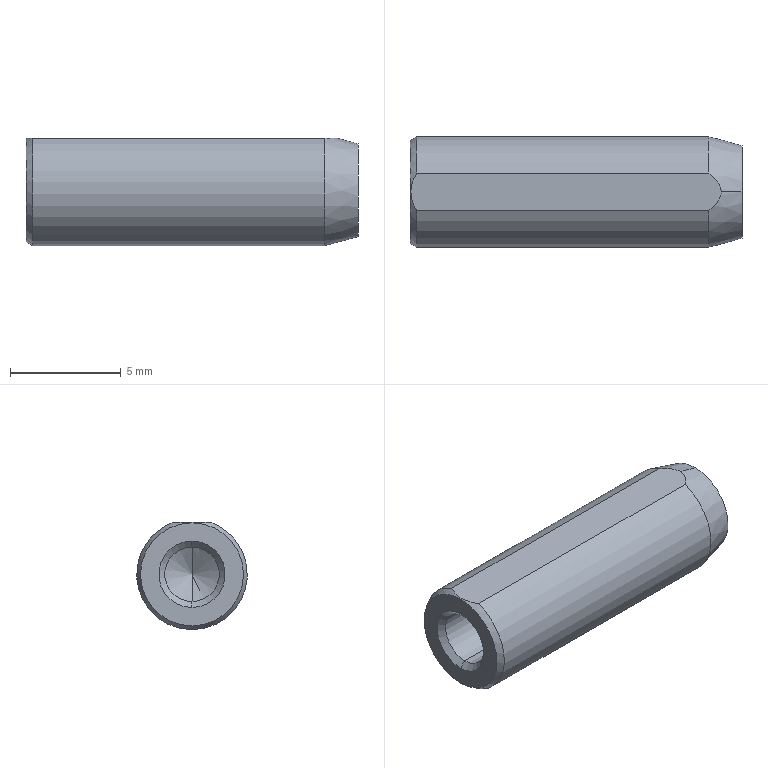Part | STEP file | MSTMS5-15-6 | 1 solid | 15 faces | box 15 x 5 x 4.85 mm | volume 252.224 mm3 | cone 8 | cylinder 4 | plane 3 | commonest cylinder face diameters 2.459 x2 5 x2
STEP:
#1=CARTESIAN_POINT('',(0.,0.,0.));
#2=DIRECTION('',(0.,0.,1.));
#3=DIRECTION('',(1.,0.,0.));
#4=AXIS2_PLACEMENT_3D('',#1,#2,#3);
#5=CARTESIAN_POINT('',(-0.4099,0.,1.23));
#6=VERTEX_POINT('',#5);
#7=CARTESIAN_POINT('',(-0.4099,0.,-1.23));
#8=VERTEX_POINT('',#7);
#9=CARTESIAN_POINT('',(-0.4099,0.,0.));
#10=DIRECTION('',(1.,0.,0.));
#11=DIRECTION('',(0.,0.,-1.));
#12=AXIS2_PLACEMENT_3D('',#9,#10,#11);
#13=CIRCLE('',#12,1.23);
#14=CARTESIAN_POINT('',(-0.4099,0.,0.));
#15=DIRECTION('',(-1.,0.,0.));
#16=DIRECTION('',(0.,0.,1.));
#17=AXIS2_PLACEMENT_3D('',#14,#15,#16);
#18=CONICAL_SURFACE('',#17,1.23,1.047);
#19=CARTESIAN_POINT('',(9.425,0.));
#20=DIRECTION('',(-1.,0.));
#21=VECTOR('',#20,1.);
#22=LINE('',#19,#21);
#23=(GEOMETRIC_REPRESENTATION_CONTEXT(2)PARAMETRIC_REPRESENTATION_CONTEXT()REPRESENTATION_CONTEXT('',''));
#24=DEFINITIONAL_REPRESENTATION('',(#22),#23);
#25=PCURVE('',#18,#24);
#26=CARTESIAN_POINT('',(0.3,0.,0.));
#27=DIRECTION('',(1.,0.,0.));
#28=DIRECTION('',(0.,0.,-1.));
#29=AXIS2_PLACEMENT_3D('',#26,#27,#28);
#30=CYLINDRICAL_SURFACE('',#29,1.23);
#31=CARTESIAN_POINT('',(0.,-0.7099));
#32=DIRECTION('',(1.,0.));
#33=VECTOR('',#32,1.);
#34=LINE('',#31,#33);
#35=(GEOMETRIC_REPRESENTATION_CONTEXT(2)PARAMETRIC_REPRESENTATION_CONTEXT()REPRESENTATION_CONTEXT('',''));
#36=DEFINITIONAL_REPRESENTATION('',(#34),#35);
#37=PCURVE('',#30,#36);
#38=SURFACE_CURVE('',#13,(#25,#37),.PCURVE_S1.);
#39=EDGE_CURVE('',#6,#8,#38,.T.);
#40=ORIENTED_EDGE('',*,*,#39,.T.);
#41=CARTESIAN_POINT('',(0.3,0.,0.));
#42=VERTEX_POINT('',#41);
#43=CARTESIAN_POINT('',(-0.4099,0.,-1.23));
#44=DIRECTION('',(-0.5,0.,-0.866));
#45=VECTOR('',#44,1.);
#46=LINE('',#43,#45);
#47=CARTESIAN_POINT('',(3.142,0.));
#48=DIRECTION('',(0.,1.));
#49=VECTOR('',#48,1.);
#50=LINE('',#47,#49);
#51=(GEOMETRIC_REPRESENTATION_CONTEXT(2)PARAMETRIC_REPRESENTATION_CONTEXT()REPRESENTATION_CONTEXT('',''));
#52=DEFINITIONAL_REPRESENTATION('',(#50),#51);
#53=PCURVE('',#18,#52);
#54=CARTESIAN_POINT('',(-0.4099,0.,0.));
#55=DIRECTION('',(-1.,0.,0.));
#56=DIRECTION('',(0.,0.,1.));
#57=AXIS2_PLACEMENT_3D('',#54,#55,#56);
#58=CONICAL_SURFACE('',#57,1.23,1.047);
#59=CARTESIAN_POINT('',(3.142,0.));
#60=DIRECTION('',(0.,1.));
#61=VECTOR('',#60,1.);
#62=LINE('',#59,#61);
#63=(GEOMETRIC_REPRESENTATION_CONTEXT(2)PARAMETRIC_REPRESENTATION_CONTEXT()REPRESENTATION_CONTEXT('',''));
#64=DEFINITIONAL_REPRESENTATION('',(#62),#63);
#65=PCURVE('',#58,#64);
#66=SURFACE_CURVE('',#46,(#53,#65),.PCURVE_S1.);
#67=EDGE_CURVE('',#42,#8,#66,.T.);
#68=ORIENTED_EDGE('',*,*,#67,.F.);
#69=CARTESIAN_POINT('',(-0.4099,0.,1.23));
#70=DIRECTION('',(-0.5,0.,0.866));
#71=VECTOR('',#70,1.);
#72=LINE('',#69,#71);
#73=CARTESIAN_POINT('',(6.283,0.));
#74=DIRECTION('',(0.,1.));
#75=VECTOR('',#74,1.);
#76=LINE('',#73,#75);
#77=(GEOMETRIC_REPRESENTATION_CONTEXT(2)PARAMETRIC_REPRESENTATION_CONTEXT()REPRESENTATION_CONTEXT('',''));
#78=DEFINITIONAL_REPRESENTATION('',(#76),#77);
#79=PCURVE('',#18,#78);
#80=CARTESIAN_POINT('',(0.,0.));
#81=DIRECTION('',(0.,1.));
#82=VECTOR('',#81,1.);
#83=LINE('',#80,#82);
#84=(GEOMETRIC_REPRESENTATION_CONTEXT(2)PARAMETRIC_REPRESENTATION_CONTEXT()REPRESENTATION_CONTEXT('',''));
#85=DEFINITIONAL_REPRESENTATION('',(#83),#84);
#86=PCURVE('',#58,#85);
#87=SURFACE_CURVE('',#72,(#79,#86),.PCURVE_S1.);
#88=EDGE_CURVE('',#42,#6,#87,.T.);
#89=ORIENTED_EDGE('',*,*,#88,.T.);
#90=EDGE_LOOP('',(#40,#68,#89));
#91=FACE_BOUND('',#90,.F.);
#92=ADVANCED_FACE('',(#91),#18,.F.);
#93=CARTESIAN_POINT('',(-7.229,0.,-1.23));
#94=VERTEX_POINT('',#93);
#95=CARTESIAN_POINT('',(0.3,0.,-1.23));
#96=DIRECTION('',(1.,0.,0.));
#97=VECTOR('',#96,1.);
#98=LINE('',#95,#97);
#99=CARTESIAN_POINT('',(6.283,0.));
#100=DIRECTION('',(0.,1.));
#101=VECTOR('',#100,1.);
#102=LINE('',#99,#101);
#103=(GEOMETRIC_REPRESENTATION_CONTEXT(2)PARAMETRIC_REPRESENTATION_CONTEXT()REPRESENTATION_CONTEXT('',''));
#104=DEFINITIONAL_REPRESENTATION('',(#102),#103);
#105=PCURVE('',#30,#104);
#106=CARTESIAN_POINT('',(0.3,0.,0.));
#107=DIRECTION('',(1.,0.,0.));
#108=DIRECTION('',(0.,0.,-1.));
#109=AXIS2_PLACEMENT_3D('',#106,#107,#108);
#110=CYLINDRICAL_SURFACE('',#109,1.23);
#111=CARTESIAN_POINT('',(0.,0.));
#112=DIRECTION('',(0.,1.));
#113=VECTOR('',#112,1.);
#114=LINE('',#111,#113);
#115=(GEOMETRIC_REPRESENTATION_CONTEXT(2)PARAMETRIC_REPRESENTATION_CONTEXT()REPRESENTATION_CONTEXT('',''));
#116=DEFINITIONAL_REPRESENTATION('',(#114),#115);
#117=PCURVE('',#110,#116);
#118=SURFACE_CURVE('',#98,(#105,#117),.PCURVE_S1.);
#119=EDGE_CURVE('',#94,#8,#118,.T.);
#120=ORIENTED_EDGE('',*,*,#119,.T.);
#121=ORIENTED_EDGE('',*,*,#39,.F.);
#122=CARTESIAN_POINT('',(-7.229,0.,1.23));
#123=VERTEX_POINT('',#122);
#124=CARTESIAN_POINT('',(0.3,0.,1.23));
#125=DIRECTION('',(1.,0.,0.));
#126=VECTOR('',#125,1.);
#127=LINE('',#124,#126);
#128=CARTESIAN_POINT('',(3.142,0.));
#129=DIRECTION('',(0.,1.));
#130=VECTOR('',#129,1.);
#131=LINE('',#128,#130);
#132=(GEOMETRIC_REPRESENTATION_CONTEXT(2)PARAMETRIC_REPRESENTATION_CONTEXT()REPRESENTATION_CONTEXT('',''));
#133=DEFINITIONAL_REPRESENTATION('',(#131),#132);
#134=PCURVE('',#30,#133);
#135=CARTESIAN_POINT('',(3.142,0.));
#136=DIRECTION('',(0.,1.));
#137=VECTOR('',#136,1.);
#138=LINE('',#135,#137);
#139=(GEOMETRIC_REPRESENTATION_CONTEXT(2)PARAMETRIC_REPRESENTATION_CONTEXT()REPRESENTATION_CONTEXT('',''));
#140=DEFINITIONAL_REPRESENTATION('',(#138),#139);
#141=PCURVE('',#110,#140);
#142=SURFACE_CURVE('',#127,(#134,#141),.PCURVE_S1.);
#143=EDGE_CURVE('',#123,#6,#142,.T.);
#144=ORIENTED_EDGE('',*,*,#143,.F.);
#145=CARTESIAN_POINT('',(-7.229,0.,0.));
#146=DIRECTION('',(1.,0.,0.));
#147=DIRECTION('',(0.,0.,-1.));
#148=AXIS2_PLACEMENT_3D('',#145,#146,#147);
#149=CIRCLE('',#148,1.23);
#150=CARTESIAN_POINT('',(0.,-7.529));
#151=DIRECTION('',(1.,0.));
#152=VECTOR('',#151,1.);
#153=LINE('',#150,#152);
#154=(GEOMETRIC_REPRESENTATION_CONTEXT(2)PARAMETRIC_REPRESENTATION_CONTEXT()REPRESENTATION_CONTEXT('',''));
#155=DEFINITIONAL_REPRESENTATION('',(#153),#154);
#156=PCURVE('',#30,#155);
#157=CARTESIAN_POINT('',(-7.5,0.,0.));
#158=DIRECTION('',(-1.,0.,0.));
#159=DIRECTION('',(0.,0.,1.));
#160=AXIS2_PLACEMENT_3D('',#157,#158,#159);
#161=CONICAL_SURFACE('',#160,1.5,0.7854);
#162=CARTESIAN_POINT('',(9.425,-0.2705));
#163=DIRECTION('',(-1.,0.));
#164=VECTOR('',#163,1.);
#165=LINE('',#162,#164);
#166=(GEOMETRIC_REPRESENTATION_CONTEXT(2)PARAMETRIC_REPRESENTATION_CONTEXT()REPRESENTATION_CONTEXT('',''));
#167=DEFINITIONAL_REPRESENTATION('',(#165),#166);
#168=PCURVE('',#161,#167);
#169=SURFACE_CURVE('',#149,(#156,#168),.PCURVE_S1.);
#170=EDGE_CURVE('',#123,#94,#169,.T.);
#171=ORIENTED_EDGE('',*,*,#170,.T.);
#172=EDGE_LOOP('',(#120,#121,#144,#171));
#173=FACE_BOUND('',#172,.F.);
#174=ADVANCED_FACE('',(#173),#30,.F.);
#175=CARTESIAN_POINT('',(-7.5,0.,1.5));
#176=VERTEX_POINT('',#175);
#177=CARTESIAN_POINT('',(-7.5,0.,1.5));
#178=DIRECTION('',(-0.7071,0.,0.7071));
#179=VECTOR('',#178,1.);
#180=LINE('',#177,#179);
#181=CARTESIAN_POINT('',(6.283,0.));
#182=DIRECTION('',(0.,1.));
#183=VECTOR('',#182,1.);
#184=LINE('',#181,#183);
#185=(GEOMETRIC_REPRESENTATION_CONTEXT(2)PARAMETRIC_REPRESENTATION_CONTEXT()REPRESENTATION_CONTEXT('',''));
#186=DEFINITIONAL_REPRESENTATION('',(#184),#185);
#187=PCURVE('',#161,#186);
#188=CARTESIAN_POINT('',(-7.5,0.,0.));
#189=DIRECTION('',(-1.,0.,0.));
#190=DIRECTION('',(0.,0.,1.));
#191=AXIS2_PLACEMENT_3D('',#188,#189,#190);
#192=CONICAL_SURFACE('',#191,1.5,0.7854);
#193=CARTESIAN_POINT('',(0.,0.));
#194=DIRECTION('',(0.,1.));
#195=VECTOR('',#194,1.);
#196=LINE('',#193,#195);
#197=(GEOMETRIC_REPRESENTATION_CONTEXT(2)PARAMETRIC_REPRESENTATION_CONTEXT()REPRESENTATION_CONTEXT('',''));
#198=DEFINITIONAL_REPRESENTATION('',(#196),#197);
#199=PCURVE('',#192,#198);
#200=SURFACE_CURVE('',#180,(#187,#199),.PCURVE_S1.);
#201=EDGE_CURVE('',#123,#176,#200,.T.);
#202=ORIENTED_EDGE('',*,*,#201,.T.);
#203=CARTESIAN_POINT('',(-7.5,0.,-1.5));
#204=VERTEX_POINT('',#203);
#205=CARTESIAN_POINT('',(-7.5,0.,0.));
#206=DIRECTION('',(1.,0.,0.));
#207=DIRECTION('',(0.,0.,-1.));
#208=AXIS2_PLACEMENT_3D('',#205,#206,#207);
#209=CIRCLE('',#208,1.5);
#210=CARTESIAN_POINT('',(9.425,0.));
#211=DIRECTION('',(-1.,0.));
#212=VECTOR('',#211,1.);
#213=LINE('',#210,#212);
#214=(GEOMETRIC_REPRESENTATION_CONTEXT(2)PARAMETRIC_REPRESENTATION_CONTEXT()REPRESENTATION_CONTEXT('',''));
#215=DEFINITIONAL_REPRESENTATION('',(#213),#214);
#216=PCURVE('',#161,#215);
#217=CARTESIAN_POINT('',(-7.5,0.,0.));
#218=DIRECTION('',(1.,0.,0.));
#219=DIRECTION('',(0.,0.,-1.));
#220=AXIS2_PLACEMENT_3D('',#217,#218,#219);
#221=PLANE('',#220);
#222=CARTESIAN_POINT('',(0.,0.));
#223=DIRECTION('',(1.,0.));
#224=AXIS2_PLACEMENT_2D('',#222,#223);
#225=CIRCLE('',#224,1.5);
#226=(GEOMETRIC_REPRESENTATION_CONTEXT(2)PARAMETRIC_REPRESENTATION_CONTEXT()REPRESENTATION_CONTEXT('',''));
#227=DEFINITIONAL_REPRESENTATION('',(#225),#226);
#228=PCURVE('',#221,#227);
#229=SURFACE_CURVE('',#209,(#216,#228),.PCURVE_S1.);
#230=EDGE_CURVE('',#176,#204,#229,.T.);
#231=ORIENTED_EDGE('',*,*,#230,.T.);
#232=CARTESIAN_POINT('',(-7.5,0.,-1.5));
#233=DIRECTION('',(-0.7071,0.,-0.7071));
#234=VECTOR('',#233,1.);
#235=LINE('',#232,#234);
#236=CARTESIAN_POINT('',(3.142,0.));
#237=DIRECTION('',(0.,1.));
#238=VECTOR('',#237,1.);
#239=LINE('',#236,#238);
#240=(GEOMETRIC_REPRESENTATION_CONTEXT(2)PARAMETRIC_REPRESENTATION_CONTEXT()REPRESENTATION_CONTEXT('',''));
#241=DEFINITIONAL_REPRESENTATION('',(#239),#240);
#242=PCURVE('',#161,#241);
#243=CARTESIAN_POINT('',(3.142,0.));
#244=DIRECTION('',(0.,1.));
#245=VECTOR('',#244,1.);
#246=LINE('',#243,#245);
#247=(GEOMETRIC_REPRESENTATION_CONTEXT(2)PARAMETRIC_REPRESENTATION_CONTEXT()REPRESENTATION_CONTEXT('',''));
#248=DEFINITIONAL_REPRESENTATION('',(#246),#247);
#249=PCURVE('',#192,#248);
#250=SURFACE_CURVE('',#235,(#242,#249),.PCURVE_S1.);
#251=EDGE_CURVE('',#94,#204,#250,.T.);
#252=ORIENTED_EDGE('',*,*,#251,.F.);
#253=ORIENTED_EDGE('',*,*,#170,.F.);
#254=EDGE_LOOP('',(#202,#231,#252,#253));
#255=FACE_BOUND('',#254,.F.);
#256=ADVANCED_FACE('',(#255),#161,.F.);
#257=CARTESIAN_POINT('',(7.5,0.,-2.098));
#258=VERTEX_POINT('',#257);
#259=CARTESIAN_POINT('',(7.5,0.,2.098));
#260=VERTEX_POINT('',#259);
#261=CARTESIAN_POINT('',(7.5,0.,0.));
#262=DIRECTION('',(1.,0.,0.));
#263=DIRECTION('',(0.,0.,-1.));
#264=AXIS2_PLACEMENT_3D('',#261,#262,#263);
#265=CIRCLE('',#264,2.098);
#266=CARTESIAN_POINT('',(6.,0.,0.));
#267=DIRECTION('',(-1.,0.,0.));
#268=DIRECTION('',(0.,0.,1.));
#269=AXIS2_PLACEMENT_3D('',#266,#267,#268);
#270=CONICAL_SURFACE('',#269,2.5,0.2618);
#271=CARTESIAN_POINT('',(3.142,-1.5));
#272=DIRECTION('',(-1.,0.));
#273=VECTOR('',#272,1.);
#274=LINE('',#271,#273);
#275=(GEOMETRIC_REPRESENTATION_CONTEXT(2)PARAMETRIC_REPRESENTATION_CONTEXT()REPRESENTATION_CONTEXT('',''));
#276=DEFINITIONAL_REPRESENTATION('',(#274),#275);
#277=PCURVE('',#270,#276);
#278=CARTESIAN_POINT('',(7.5,2.098,0.));
#279=DIRECTION('',(-1.,0.,0.));
#280=DIRECTION('',(0.,0.,1.));
#281=AXIS2_PLACEMENT_3D('',#278,#279,#280);
#282=PLANE('',#281);
#283=CARTESIAN_POINT('',(-2.098,-2.098));
#284=CARTESIAN_POINT('',(-2.098,1.536));
#285=CARTESIAN_POINT('',(1.049,-0.2811));
#286=CARTESIAN_POINT('',(4.196,-2.098));
#287=CARTESIAN_POINT('',(1.049,-3.915));
#288=CARTESIAN_POINT('',(-2.098,-5.732));
#289=CARTESIAN_POINT('',(-2.098,-2.098));
#290=(BOUNDED_CURVE()B_SPLINE_CURVE(2,(#283,#284,#285,#286,#287,#288,#289),.UNSPECIFIED.,.T.,.F.)B_SPLINE_CURVE_WITH_KNOTS((1,2,2,2,2,1),(-2.094,0.,2.094,4.189,6.283,8.378),.UNSPECIFIED.)CURVE()GEOMETRIC_REPRESENTATION_ITEM()RATIONAL_B_SPLINE_CURVE((1.,0.5,1.,0.5,1.,0.5,1.))REPRESENTATION_ITEM(''));
#291=(GEOMETRIC_REPRESENTATION_CONTEXT(2)PARAMETRIC_REPRESENTATION_CONTEXT()REPRESENTATION_CONTEXT('',''));
#292=DEFINITIONAL_REPRESENTATION('',(#290),#291);
#293=PCURVE('',#282,#292);
#294=SURFACE_CURVE('',#265,(#277,#293),.PCURVE_S1.);
#295=EDGE_CURVE('',#258,#260,#294,.T.);
#296=ORIENTED_EDGE('',*,*,#295,.F.);
#297=CARTESIAN_POINT('',(6.,0.,-2.5));
#298=VERTEX_POINT('',#297);
#299=CARTESIAN_POINT('',(6.,0.,-2.5));
#300=DIRECTION('',(-0.9659,0.,-0.2588));
#301=VECTOR('',#300,1.);
#302=LINE('',#299,#301);
#303=CARTESIAN_POINT('',(3.142,0.));
#304=DIRECTION('',(0.,1.));
#305=VECTOR('',#304,1.);
#306=LINE('',#303,#305);
#307=(GEOMETRIC_REPRESENTATION_CONTEXT(2)PARAMETRIC_REPRESENTATION_CONTEXT()REPRESENTATION_CONTEXT('',''));
#308=DEFINITIONAL_REPRESENTATION('',(#306),#307);
#309=PCURVE('',#270,#308);
#310=CARTESIAN_POINT('',(6.,0.,0.));
#311=DIRECTION('',(-1.,0.,0.));
#312=DIRECTION('',(0.,0.,1.));
#313=AXIS2_PLACEMENT_3D('',#310,#311,#312);
#314=CONICAL_SURFACE('',#313,2.5,0.2618);
#315=CARTESIAN_POINT('',(3.142,0.));
#316=DIRECTION('',(0.,1.));
#317=VECTOR('',#316,1.);
#318=LINE('',#315,#317);
#319=(GEOMETRIC_REPRESENTATION_CONTEXT(2)PARAMETRIC_REPRESENTATION_CONTEXT()REPRESENTATION_CONTEXT('',''));
#320=DEFINITIONAL_REPRESENTATION('',(#318),#319);
#321=PCURVE('',#314,#320);
#322=SURFACE_CURVE('',#302,(#309,#321),.PCURVE_S1.);
#323=EDGE_CURVE('',#258,#298,#322,.T.);
#324=ORIENTED_EDGE('',*,*,#323,.T.);
#325=CARTESIAN_POINT('',(6.,0.8529,2.35));
#326=VERTEX_POINT('',#325);
#327=CARTESIAN_POINT('',(6.,0.,0.));
#328=DIRECTION('',(1.,0.,0.));
#329=DIRECTION('',(0.,0.,-1.));
#330=AXIS2_PLACEMENT_3D('',#327,#328,#329);
#331=CIRCLE('',#330,2.5);
#332=CARTESIAN_POINT('',(3.142,0.));
#333=DIRECTION('',(-1.,0.));
#334=VECTOR('',#333,1.);
#335=LINE('',#332,#334);
#336=(GEOMETRIC_REPRESENTATION_CONTEXT(2)PARAMETRIC_REPRESENTATION_CONTEXT()REPRESENTATION_CONTEXT('',''));
#337=DEFINITIONAL_REPRESENTATION('',(#335),#336);
#338=PCURVE('',#270,#337);
#339=CARTESIAN_POINT('',(7.5,0.,0.));
#340=DIRECTION('',(1.,0.,0.));
#341=DIRECTION('',(0.,0.,-1.));
#342=AXIS2_PLACEMENT_3D('',#339,#340,#341);
#343=CYLINDRICAL_SURFACE('',#342,2.5);
#344=CARTESIAN_POINT('',(0.,-1.5));
#345=DIRECTION('',(1.,0.));
#346=VECTOR('',#345,1.);
#347=LINE('',#344,#346);
#348=(GEOMETRIC_REPRESENTATION_CONTEXT(2)PARAMETRIC_REPRESENTATION_CONTEXT()REPRESENTATION_CONTEXT('',''));
#349=DEFINITIONAL_REPRESENTATION('',(#347),#348);
#350=PCURVE('',#343,#349);
#351=SURFACE_CURVE('',#331,(#338,#350),.PCURVE_S1.);
#352=EDGE_CURVE('',#298,#326,#351,.T.);
#353=ORIENTED_EDGE('',*,*,#352,.T.);
#354=CARTESIAN_POINT('',(6.56,0.,2.35));
#355=VERTEX_POINT('',#354);
#356=CARTESIAN_POINT('',(6.56,0.,2.35));
#357=CARTESIAN_POINT('',(6.56,0.08831,2.35));
#358=CARTESIAN_POINT('',(6.541,0.176,2.35));
#359=CARTESIAN_POINT('',(6.473,0.3408,2.35));
#360=CARTESIAN_POINT('',(6.427,0.4157,2.35));
#361=CARTESIAN_POINT('',(6.268,0.6265,2.35));
#362=CARTESIAN_POINT('',(6.137,0.7453,2.35));
#363=CARTESIAN_POINT('',(6.,0.8529,2.35));
#364=B_SPLINE_CURVE_WITH_KNOTS('',3,(#356,#357,#358,#359,#360,#361,#362,#363),.UNSPECIFIED.,.F.,.F.,(4,2,2,4),(0.006758,0.007021,0.007285,0.007811),.UNSPECIFIED.);
#365=CARTESIAN_POINT('',(0.,-0.5598));
#366=CARTESIAN_POINT('',(0.006833,-0.5598));
#367=CARTESIAN_POINT('',(0.02048,-0.5585));
#368=CARTESIAN_POINT('',(0.04081,-0.553));
#369=CARTESIAN_POINT('',(0.06091,-0.544));
#370=CARTESIAN_POINT('',(0.08069,-0.5317));
#371=CARTESIAN_POINT('',(0.1001,-0.5163));
#372=CARTESIAN_POINT('',(0.119,-0.4979));
#373=CARTESIAN_POINT('',(0.1372,-0.4772));
#374=CARTESIAN_POINT('',(0.1548,-0.4543));
#375=CARTESIAN_POINT('',(0.1717,-0.4294));
#376=CARTESIAN_POINT('',(0.1881,-0.4027));
#377=CARTESIAN_POINT('',(0.204,-0.3745));
#378=CARTESIAN_POINT('',(0.2194,-0.3448));
#379=CARTESIAN_POINT('',(0.2342,-0.3141));
#380=CARTESIAN_POINT('',(0.2486,-0.2823));
#381=CARTESIAN_POINT('',(0.2625,-0.2496));
#382=CARTESIAN_POINT('',(0.2759,-0.2159));
#383=CARTESIAN_POINT('',(0.2889,-0.1814));
#384=CARTESIAN_POINT('',(0.3015,-0.1463));
#385=CARTESIAN_POINT('',(0.3137,-0.1105));
#386=CARTESIAN_POINT('',(0.3255,-0.0741));
#387=CARTESIAN_POINT('',(0.337,-0.03727));
#388=CARTESIAN_POINT('',(0.3445,-0.01246));
#389=CARTESIAN_POINT('',(0.3482,0.));
#390=B_SPLINE_CURVE_WITH_KNOTS('',3,(#365,#366,#367,#368,#369,#370,#371,#372,#373,#374,#375,#376,#377,#378,#379,#380,#381,#382,#383,#384,#385,#386,#387,#388,#389),.UNSPECIFIED.,.F.,.F.,(4,1,1,1,1,1,1,1,1,1,1,1,1,1,1,1,1,1,1,1,1,1,4),(0.006758,0.006806,0.006854,0.006902,0.00695,0.006997,0.007045,0.007093,0.007141,0.007189,0.007237,0.007285,0.007332,0.00738,0.007428,0.007476,0.007524,0.007572,0.00762,0.007667,0.007715,0.007763,0.007811),.QUASI_UNIFORM_KNOTS.);
#391=(GEOMETRIC_REPRESENTATION_CONTEXT(2)PARAMETRIC_REPRESENTATION_CONTEXT()REPRESENTATION_CONTEXT('',''));
#392=DEFINITIONAL_REPRESENTATION('',(#390),#391);
#393=PCURVE('',#270,#392);
#394=CARTESIAN_POINT('',(7.5,-2.5,2.35));
#395=DIRECTION('',(0.,0.,1.));
#396=DIRECTION('',(1.,0.,0.));
#397=AXIS2_PLACEMENT_3D('',#394,#395,#396);
#398=PLANE('',#397);
#399=CARTESIAN_POINT('',(-0.9402,2.5));
#400=CARTESIAN_POINT('',(-0.9402,2.588));
#401=CARTESIAN_POINT('',(-0.9594,2.676));
#402=CARTESIAN_POINT('',(-1.027,2.841));
#403=CARTESIAN_POINT('',(-1.073,2.916));
#404=CARTESIAN_POINT('',(-1.232,3.127));
#405=CARTESIAN_POINT('',(-1.363,3.245));
#406=CARTESIAN_POINT('',(-1.5,3.353));
#407=B_SPLINE_CURVE_WITH_KNOTS('',3,(#399,#400,#401,#402,#403,#404,#405,#406),.UNSPECIFIED.,.F.,.F.,(4,2,2,4),(0.006758,0.007021,0.007285,0.007811),.UNSPECIFIED.);
#408=(GEOMETRIC_REPRESENTATION_CONTEXT(2)PARAMETRIC_REPRESENTATION_CONTEXT()REPRESENTATION_CONTEXT('',''));
#409=DEFINITIONAL_REPRESENTATION('',(#407),#408);
#410=PCURVE('',#398,#409);
#411=SURFACE_CURVE('',#364,(#393,#410),.PCURVE_S1.);
#412=EDGE_CURVE('',#355,#326,#411,.T.);
#413=ORIENTED_EDGE('',*,*,#412,.F.);
#414=CARTESIAN_POINT('',(6.,0.,2.5));
#415=DIRECTION('',(-0.9659,0.,0.2588));
#416=VECTOR('',#415,1.);
#417=LINE('',#414,#416);
#418=CARTESIAN_POINT('',(0.,0.));
#419=DIRECTION('',(0.,1.));
#420=VECTOR('',#419,1.);
#421=LINE('',#418,#420);
#422=(GEOMETRIC_REPRESENTATION_CONTEXT(2)PARAMETRIC_REPRESENTATION_CONTEXT()REPRESENTATION_CONTEXT('',''));
#423=DEFINITIONAL_REPRESENTATION('',(#421),#422);
#424=PCURVE('',#270,#423);
#425=CARTESIAN_POINT('',(6.283,0.));
#426=DIRECTION('',(0.,1.));
#427=VECTOR('',#426,1.);
#428=LINE('',#425,#427);
#429=(GEOMETRIC_REPRESENTATION_CONTEXT(2)PARAMETRIC_REPRESENTATION_CONTEXT()REPRESENTATION_CONTEXT('',''));
#430=DEFINITIONAL_REPRESENTATION('',(#428),#429);
#431=PCURVE('',#314,#430);
#432=SURFACE_CURVE('',#417,(#424,#431),.PCURVE_S1.);
#433=EDGE_CURVE('',#260,#355,#432,.T.);
#434=ORIENTED_EDGE('',*,*,#433,.F.);
#435=EDGE_LOOP('',(#296,#324,#353,#413,#434));
#436=FACE_BOUND('',#435,.T.);
#437=ADVANCED_FACE('',(#436),#270,.T.);
#438=CARTESIAN_POINT('',(-7.2,-0.8529,2.35));
#439=VERTEX_POINT('',#438);
#440=CARTESIAN_POINT('',(-7.2,0.,-2.5));
#441=VERTEX_POINT('',#440);
#442=CARTESIAN_POINT('',(-7.2,0.,0.));
#443=DIRECTION('',(1.,0.,0.));
#444=DIRECTION('',(0.,0.,-1.));
#445=AXIS2_PLACEMENT_3D('',#442,#443,#444);
#446=CIRCLE('',#445,2.5);
#447=CARTESIAN_POINT('',(7.5,0.,0.));
#448=DIRECTION('',(1.,0.,0.));
#449=DIRECTION('',(0.,0.,-1.));
#450=AXIS2_PLACEMENT_3D('',#447,#448,#449);
#451=CYLINDRICAL_SURFACE('',#450,2.5);
#452=CARTESIAN_POINT('',(0.,-14.7));
#453=DIRECTION('',(1.,0.));
#454=VECTOR('',#453,1.);
#455=LINE('',#452,#454);
#456=(GEOMETRIC_REPRESENTATION_CONTEXT(2)PARAMETRIC_REPRESENTATION_CONTEXT()REPRESENTATION_CONTEXT('',''));
#457=DEFINITIONAL_REPRESENTATION('',(#455),#456);
#458=PCURVE('',#451,#457);
#459=CARTESIAN_POINT('',(-7.5,0.,0.));
#460=DIRECTION('',(1.,0.,0.));
#461=DIRECTION('',(0.,0.,-1.));
#462=AXIS2_PLACEMENT_3D('',#459,#460,#461);
#463=CONICAL_SURFACE('',#462,2.327,0.5236);
#464=CARTESIAN_POINT('',(0.,0.3));
#465=DIRECTION('',(1.,0.));
#466=VECTOR('',#465,1.);
#467=LINE('',#464,#466);
#468=(GEOMETRIC_REPRESENTATION_CONTEXT(2)PARAMETRIC_REPRESENTATION_CONTEXT()REPRESENTATION_CONTEXT('',''));
#469=DEFINITIONAL_REPRESENTATION('',(#467),#468);
#470=PCURVE('',#463,#469);
#471=SURFACE_CURVE('',#446,(#458,#470),.PCURVE_S1.);
#472=EDGE_CURVE('',#439,#441,#471,.T.);
#473=ORIENTED_EDGE('',*,*,#472,.T.);
#474=CARTESIAN_POINT('',(7.5,0.,-2.5));
#475=DIRECTION('',(1.,0.,0.));
#476=VECTOR('',#475,1.);
#477=LINE('',#474,#476);
#478=CARTESIAN_POINT('',(6.283,0.));
#479=DIRECTION('',(0.,1.));
#480=VECTOR('',#479,1.);
#481=LINE('',#478,#480);
#482=(GEOMETRIC_REPRESENTATION_CONTEXT(2)PARAMETRIC_REPRESENTATION_CONTEXT()REPRESENTATION_CONTEXT('',''));
#483=DEFINITIONAL_REPRESENTATION('',(#481),#482);
#484=PCURVE('',#451,#483);
#485=CARTESIAN_POINT('',(0.,0.));
#486=DIRECTION('',(0.,1.));
#487=VECTOR('',#486,1.);
#488=LINE('',#485,#487);
#489=(GEOMETRIC_REPRESENTATION_CONTEXT(2)PARAMETRIC_REPRESENTATION_CONTEXT()REPRESENTATION_CONTEXT('',''));
#490=DEFINITIONAL_REPRESENTATION('',(#488),#489);
#491=PCURVE('',#343,#490);
#492=SURFACE_CURVE('',#477,(#484,#491),.PCURVE_S1.);
#493=EDGE_CURVE('',#441,#298,#492,.T.);
#494=ORIENTED_EDGE('',*,*,#493,.T.);
#495=CARTESIAN_POINT('',(6.,-0.8529,2.35));
#496=VERTEX_POINT('',#495);
#497=CARTESIAN_POINT('',(6.,0.,0.));
#498=DIRECTION('',(1.,0.,0.));
#499=DIRECTION('',(0.,0.,-1.));
#500=AXIS2_PLACEMENT_3D('',#497,#498,#499);
#501=CIRCLE('',#500,2.5);
#502=CARTESIAN_POINT('',(0.,-1.5));
#503=DIRECTION('',(1.,0.));
#504=VECTOR('',#503,1.);
#505=LINE('',#502,#504);
#506=(GEOMETRIC_REPRESENTATION_CONTEXT(2)PARAMETRIC_REPRESENTATION_CONTEXT()REPRESENTATION_CONTEXT('',''));
#507=DEFINITIONAL_REPRESENTATION('',(#505),#506);
#508=PCURVE('',#451,#507);
#509=CARTESIAN_POINT('',(9.425,0.));
#510=DIRECTION('',(-1.,0.));
#511=VECTOR('',#510,1.);
#512=LINE('',#509,#511);
#513=(GEOMETRIC_REPRESENTATION_CONTEXT(2)PARAMETRIC_REPRESENTATION_CONTEXT()REPRESENTATION_CONTEXT('',''));
#514=DEFINITIONAL_REPRESENTATION('',(#512),#513);
#515=PCURVE('',#314,#514);
#516=SURFACE_CURVE('',#501,(#508,#515),.PCURVE_S1.);
#517=EDGE_CURVE('',#496,#298,#516,.T.);
#518=ORIENTED_EDGE('',*,*,#517,.F.);
#519=CARTESIAN_POINT('',(7.5,-0.8529,2.35));
#520=DIRECTION('',(1.,0.,0.));
#521=VECTOR('',#520,1.);
#522=LINE('',#519,#521);
#523=CARTESIAN_POINT('',(3.49,0.));
#524=DIRECTION('',(0.,1.));
#525=VECTOR('',#524,1.);
#526=LINE('',#523,#525);
#527=(GEOMETRIC_REPRESENTATION_CONTEXT(2)PARAMETRIC_REPRESENTATION_CONTEXT()REPRESENTATION_CONTEXT('',''));
#528=DEFINITIONAL_REPRESENTATION('',(#526),#527);
#529=PCURVE('',#451,#528);
#530=CARTESIAN_POINT('',(0.,1.647));
#531=DIRECTION('',(1.,0.));
#532=VECTOR('',#531,1.);
#533=LINE('',#530,#532);
#534=(GEOMETRIC_REPRESENTATION_CONTEXT(2)PARAMETRIC_REPRESENTATION_CONTEXT()REPRESENTATION_CONTEXT('',''));
#535=DEFINITIONAL_REPRESENTATION('',(#533),#534);
#536=PCURVE('',#398,#535);
#537=SURFACE_CURVE('',#522,(#529,#536),.PCURVE_S1.);
#538=EDGE_CURVE('',#439,#496,#537,.T.);
#539=ORIENTED_EDGE('',*,*,#538,.F.);
#540=EDGE_LOOP('',(#473,#494,#518,#539));
#541=FACE_BOUND('',#540,.T.);
#542=ADVANCED_FACE('',(#541),#451,.T.);
#543=CARTESIAN_POINT('',(-7.5,0.,-2.327));
#544=VERTEX_POINT('',#543);
#545=CARTESIAN_POINT('',(-7.5,0.,2.327));
#546=VERTEX_POINT('',#545);
#547=CARTESIAN_POINT('',(-7.5,0.,0.));
#548=DIRECTION('',(1.,0.,0.));
#549=DIRECTION('',(0.,0.,-1.));
#550=AXIS2_PLACEMENT_3D('',#547,#548,#549);
#551=CIRCLE('',#550,2.327);
#552=CARTESIAN_POINT('',(-7.5,0.,0.));
#553=DIRECTION('',(1.,0.,0.));
#554=DIRECTION('',(0.,0.,-1.));
#555=AXIS2_PLACEMENT_3D('',#552,#553,#554);
#556=CONICAL_SURFACE('',#555,2.327,0.5236);
#557=CARTESIAN_POINT('',(0.,0.));
#558=DIRECTION('',(1.,0.));
#559=VECTOR('',#558,1.);
#560=LINE('',#557,#559);
#561=(GEOMETRIC_REPRESENTATION_CONTEXT(2)PARAMETRIC_REPRESENTATION_CONTEXT()REPRESENTATION_CONTEXT('',''));
#562=DEFINITIONAL_REPRESENTATION('',(#560),#561);
#563=PCURVE('',#556,#562);
#564=CARTESIAN_POINT('',(0.,0.));
#565=DIRECTION('',(1.,0.));
#566=AXIS2_PLACEMENT_2D('',#564,#565);
#567=CIRCLE('',#566,2.327);
#568=(GEOMETRIC_REPRESENTATION_CONTEXT(2)PARAMETRIC_REPRESENTATION_CONTEXT()REPRESENTATION_CONTEXT('',''));
#569=DEFINITIONAL_REPRESENTATION('',(#567),#568);
#570=PCURVE('',#221,#569);
#571=SURFACE_CURVE('',#551,(#563,#570),.PCURVE_S1.);
#572=EDGE_CURVE('',#544,#546,#571,.T.);
#573=ORIENTED_EDGE('',*,*,#572,.T.);
#574=CARTESIAN_POINT('',(-7.46,0.,2.35));
#575=VERTEX_POINT('',#574);
#576=CARTESIAN_POINT('',(-7.5,0.,2.327));
#577=DIRECTION('',(0.866,0.,0.5));
#578=VECTOR('',#577,1.);
#579=LINE('',#576,#578);
#580=CARTESIAN_POINT('',(3.142,0.));
#581=DIRECTION('',(0.,1.));
#582=VECTOR('',#581,1.);
#583=LINE('',#580,#582);
#584=(GEOMETRIC_REPRESENTATION_CONTEXT(2)PARAMETRIC_REPRESENTATION_CONTEXT()REPRESENTATION_CONTEXT('',''));
#585=DEFINITIONAL_REPRESENTATION('',(#583),#584);
#586=PCURVE('',#556,#585);
#587=CARTESIAN_POINT('',(3.142,0.));
#588=DIRECTION('',(0.,1.));
#589=VECTOR('',#588,1.);
#590=LINE('',#587,#589);
#591=(GEOMETRIC_REPRESENTATION_CONTEXT(2)PARAMETRIC_REPRESENTATION_CONTEXT()REPRESENTATION_CONTEXT('',''));
#592=DEFINITIONAL_REPRESENTATION('',(#590),#591);
#593=PCURVE('',#463,#592);
#594=SURFACE_CURVE('',#579,(#586,#593),.PCURVE_S1.);
#595=EDGE_CURVE('',#546,#575,#594,.T.);
#596=ORIENTED_EDGE('',*,*,#595,.T.);
#597=CARTESIAN_POINT('',(-7.2,0.8529,2.35));
#598=VERTEX_POINT('',#597);
#599=CARTESIAN_POINT('',(-7.2,0.8529,2.35));
#600=CARTESIAN_POINT('',(-7.276,0.7245,2.35));
#601=CARTESIAN_POINT('',(-7.342,0.5874,2.35));
#602=CARTESIAN_POINT('',(-7.434,0.3007,2.35));
#603=CARTESIAN_POINT('',(-7.46,0.151,2.35));
#604=CARTESIAN_POINT('',(-7.46,0.,2.35));
#605=B_SPLINE_CURVE_WITH_KNOTS('',3,(#599,#600,#601,#602,#603,#604),.UNSPECIFIED.,.F.,.F.,(4,2,4),(0.006451,0.006901,0.007351),.UNSPECIFIED.);
#606=CARTESIAN_POINT('',(2.793,0.3));
#607=CARTESIAN_POINT('',(2.798,0.2931));
#608=CARTESIAN_POINT('',(2.807,0.2795));
#609=CARTESIAN_POINT('',(2.82,0.2596));
#610=CARTESIAN_POINT('',(2.834,0.2402));
#611=CARTESIAN_POINT('',(2.848,0.2215));
#612=CARTESIAN_POINT('',(2.863,0.2035));
#613=CARTESIAN_POINT('',(2.877,0.1862));
#614=CARTESIAN_POINT('',(2.892,0.1697));
#615=CARTESIAN_POINT('',(2.908,0.154));
#616=CARTESIAN_POINT('',(2.923,0.1391));
#617=CARTESIAN_POINT('',(2.939,0.1251));
#618=CARTESIAN_POINT('',(2.955,0.1121));
#619=CARTESIAN_POINT('',(2.971,0.09998));
#620=CARTESIAN_POINT('',(2.987,0.08892));
#621=CARTESIAN_POINT('',(3.004,0.07892));
#622=CARTESIAN_POINT('',(3.021,0.07));
#623=CARTESIAN_POINT('',(3.038,0.06218));
#624=CARTESIAN_POINT('',(3.055,0.0555));
#625=CARTESIAN_POINT('',(3.072,0.04998));
#626=CARTESIAN_POINT('',(3.089,0.04564));
#627=CARTESIAN_POINT('',(3.107,0.04251));
#628=CARTESIAN_POINT('',(3.124,0.04062));
#629=CARTESIAN_POINT('',(3.136,0.04019));
#630=CARTESIAN_POINT('',(3.142,0.04019));
#631=B_SPLINE_CURVE_WITH_KNOTS('',3,(#606,#607,#608,#609,#610,#611,#612,#613,#614,#615,#616,#617,#618,#619,#620,#621,#622,#623,#624,#625,#626,#627,#628,#629,#630),.UNSPECIFIED.,.F.,.F.,(4,1,1,1,1,1,1,1,1,1,1,1,1,1,1,1,1,1,1,1,1,1,4),(0.006451,0.006492,0.006533,0.006574,0.006615,0.006656,0.006697,0.006738,0.006778,0.006819,0.00686,0.006901,0.006942,0.006983,0.007024,0.007065,0.007106,0.007147,0.007188,0.007229,0.00727,0.00731,0.007351),.QUASI_UNIFORM_KNOTS.);
#632=(GEOMETRIC_REPRESENTATION_CONTEXT(2)PARAMETRIC_REPRESENTATION_CONTEXT()REPRESENTATION_CONTEXT('',''));
#633=DEFINITIONAL_REPRESENTATION('',(#631),#632);
#634=PCURVE('',#556,#633);
#635=CARTESIAN_POINT('',(-14.7,3.353));
#636=CARTESIAN_POINT('',(-14.776,3.224));
#637=CARTESIAN_POINT('',(-14.842,3.087));
#638=CARTESIAN_POINT('',(-14.934,2.801));
#639=CARTESIAN_POINT('',(-14.96,2.651));
#640=CARTESIAN_POINT('',(-14.96,2.5));
#641=B_SPLINE_CURVE_WITH_KNOTS('',3,(#635,#636,#637,#638,#639,#640),.UNSPECIFIED.,.F.,.F.,(4,2,4),(0.006451,0.006901,0.007351),.UNSPECIFIED.);
#642=(GEOMETRIC_REPRESENTATION_CONTEXT(2)PARAMETRIC_REPRESENTATION_CONTEXT()REPRESENTATION_CONTEXT('',''));
#643=DEFINITIONAL_REPRESENTATION('',(#641),#642);
#644=PCURVE('',#398,#643);
#645=SURFACE_CURVE('',#605,(#634,#644),.PCURVE_S1.);
#646=EDGE_CURVE('',#598,#575,#645,.T.);
#647=ORIENTED_EDGE('',*,*,#646,.F.);
#648=CARTESIAN_POINT('',(-7.2,0.,0.));
#649=DIRECTION('',(1.,0.,0.));
#650=DIRECTION('',(0.,0.,-1.));
#651=AXIS2_PLACEMENT_3D('',#648,#649,#650);
#652=CIRCLE('',#651,2.5);
#653=CARTESIAN_POINT('',(0.,0.3));
#654=DIRECTION('',(1.,0.));
#655=VECTOR('',#654,1.);
#656=LINE('',#653,#655);
#657=(GEOMETRIC_REPRESENTATION_CONTEXT(2)PARAMETRIC_REPRESENTATION_CONTEXT()REPRESENTATION_CONTEXT('',''));
#658=DEFINITIONAL_REPRESENTATION('',(#656),#657);
#659=PCURVE('',#556,#658);
#660=CARTESIAN_POINT('',(0.,-14.7));
#661=DIRECTION('',(1.,0.));
#662=VECTOR('',#661,1.);
#663=LINE('',#660,#662);
#664=(GEOMETRIC_REPRESENTATION_CONTEXT(2)PARAMETRIC_REPRESENTATION_CONTEXT()REPRESENTATION_CONTEXT('',''));
#665=DEFINITIONAL_REPRESENTATION('',(#663),#664);
#666=PCURVE('',#343,#665);
#667=SURFACE_CURVE('',#652,(#659,#666),.PCURVE_S1.);
#668=EDGE_CURVE('',#441,#598,#667,.T.);
#669=ORIENTED_EDGE('',*,*,#668,.F.);
#670=CARTESIAN_POINT('',(-7.5,0.,-2.327));
#671=DIRECTION('',(0.866,0.,-0.5));
#672=VECTOR('',#671,1.);
#673=LINE('',#670,#672);
#674=CARTESIAN_POINT('',(0.,0.));
#675=DIRECTION('',(0.,1.));
#676=VECTOR('',#675,1.);
#677=LINE('',#674,#676);
#678=(GEOMETRIC_REPRESENTATION_CONTEXT(2)PARAMETRIC_REPRESENTATION_CONTEXT()REPRESENTATION_CONTEXT('',''));
#679=DEFINITIONAL_REPRESENTATION('',(#677),#678);
#680=PCURVE('',#556,#679);
#681=CARTESIAN_POINT('',(6.283,0.));
#682=DIRECTION('',(0.,1.));
#683=VECTOR('',#682,1.);
#684=LINE('',#681,#683);
#685=(GEOMETRIC_REPRESENTATION_CONTEXT(2)PARAMETRIC_REPRESENTATION_CONTEXT()REPRESENTATION_CONTEXT('',''));
#686=DEFINITIONAL_REPRESENTATION('',(#684),#685);
#687=PCURVE('',#463,#686);
#688=SURFACE_CURVE('',#673,(#680,#687),.PCURVE_S1.);
#689=EDGE_CURVE('',#544,#441,#688,.T.);
#690=ORIENTED_EDGE('',*,*,#689,.F.);
#691=EDGE_LOOP('',(#573,#596,#647,#669,#690));
#692=FACE_BOUND('',#691,.T.);
#693=ADVANCED_FACE('',(#692),#556,.T.);
#694=ORIENTED_EDGE('',*,*,#595,.F.);
#695=CARTESIAN_POINT('',(-7.5,0.,0.));
#696=DIRECTION('',(1.,0.,0.));
#697=DIRECTION('',(0.,0.,-1.));
#698=AXIS2_PLACEMENT_3D('',#695,#696,#697);
#699=CIRCLE('',#698,2.327);
#700=CARTESIAN_POINT('',(0.,0.));
#701=DIRECTION('',(1.,0.));
#702=VECTOR('',#701,1.);
#703=LINE('',#700,#702);
#704=(GEOMETRIC_REPRESENTATION_CONTEXT(2)PARAMETRIC_REPRESENTATION_CONTEXT()REPRESENTATION_CONTEXT('',''));
#705=DEFINITIONAL_REPRESENTATION('',(#703),#704);
#706=PCURVE('',#463,#705);
#707=CARTESIAN_POINT('',(0.,0.));
#708=DIRECTION('',(1.,0.));
#709=AXIS2_PLACEMENT_2D('',#707,#708);
#710=CIRCLE('',#709,2.327);
#711=(GEOMETRIC_REPRESENTATION_CONTEXT(2)PARAMETRIC_REPRESENTATION_CONTEXT()REPRESENTATION_CONTEXT('',''));
#712=DEFINITIONAL_REPRESENTATION('',(#710),#711);
#713=PCURVE('',#221,#712);
#714=SURFACE_CURVE('',#699,(#706,#713),.PCURVE_S1.);
#715=EDGE_CURVE('',#546,#544,#714,.T.);
#716=ORIENTED_EDGE('',*,*,#715,.T.);
#717=ORIENTED_EDGE('',*,*,#689,.T.);
#718=ORIENTED_EDGE('',*,*,#472,.F.);
#719=CARTESIAN_POINT('',(-7.46,0.,2.35));
#720=CARTESIAN_POINT('',(-7.46,-0.1513,2.35));
#721=CARTESIAN_POINT('',(-7.434,-0.2995,2.35));
#722=CARTESIAN_POINT('',(-7.341,-0.5886,2.35));
#723=CARTESIAN_POINT('',(-7.276,-0.7237,2.35));
#724=CARTESIAN_POINT('',(-7.2,-0.8529,2.35));
#725=B_SPLINE_CURVE_WITH_KNOTS('',3,(#719,#720,#721,#722,#723,#724),.UNSPECIFIED.,.F.,.F.,(4,2,4),(0.007351,0.007802,0.008253),.UNSPECIFIED.);
#726=CARTESIAN_POINT('',(3.142,0.04019));
#727=CARTESIAN_POINT('',(3.147,0.04019));
#728=CARTESIAN_POINT('',(3.159,0.04061));
#729=CARTESIAN_POINT('',(3.177,0.04249));
#730=CARTESIAN_POINT('',(3.194,0.04559));
#731=CARTESIAN_POINT('',(3.211,0.0499));
#732=CARTESIAN_POINT('',(3.228,0.05539));
#733=CARTESIAN_POINT('',(3.245,0.06205));
#734=CARTESIAN_POINT('',(3.262,0.06985));
#735=CARTESIAN_POINT('',(3.279,0.07877));
#736=CARTESIAN_POINT('',(3.296,0.08879));
#737=CARTESIAN_POINT('',(3.312,0.09989));
#738=CARTESIAN_POINT('',(3.328,0.1121));
#739=CARTESIAN_POINT('',(3.344,0.1252));
#740=CARTESIAN_POINT('',(3.36,0.1392));
#741=CARTESIAN_POINT('',(3.376,0.1541));
#742=CARTESIAN_POINT('',(3.391,0.1698));
#743=CARTESIAN_POINT('',(3.406,0.1863));
#744=CARTESIAN_POINT('',(3.42,0.2035));
#745=CARTESIAN_POINT('',(3.435,0.2215));
#746=CARTESIAN_POINT('',(3.449,0.2401));
#747=CARTESIAN_POINT('',(3.463,0.2594));
#748=CARTESIAN_POINT('',(3.476,0.2794));
#749=CARTESIAN_POINT('',(3.485,0.2931));
#750=CARTESIAN_POINT('',(3.49,0.3));
#751=B_SPLINE_CURVE_WITH_KNOTS('',3,(#726,#727,#728,#729,#730,#731,#732,#733,#734,#735,#736,#737,#738,#739,#740,#741,#742,#743,#744,#745,#746,#747,#748,#749,#750),.UNSPECIFIED.,.F.,.F.,(4,1,1,1,1,1,1,1,1,1,1,1,1,1,1,1,1,1,1,1,1,1,4),(0.007351,0.007392,0.007433,0.007474,0.007515,0.007556,0.007597,0.007638,0.007679,0.00772,0.007761,0.007802,0.007843,0.007884,0.007925,0.007966,0.008007,0.008048,0.008089,0.00813,0.008171,0.008212,0.008253),.QUASI_UNIFORM_KNOTS.);
#752=(GEOMETRIC_REPRESENTATION_CONTEXT(2)PARAMETRIC_REPRESENTATION_CONTEXT()REPRESENTATION_CONTEXT('',''));
#753=DEFINITIONAL_REPRESENTATION('',(#751),#752);
#754=PCURVE('',#463,#753);
#755=CARTESIAN_POINT('',(-14.96,2.5));
#756=CARTESIAN_POINT('',(-14.96,2.349));
#757=CARTESIAN_POINT('',(-14.934,2.2));
#758=CARTESIAN_POINT('',(-14.841,1.911));
#759=CARTESIAN_POINT('',(-14.776,1.776));
#760=CARTESIAN_POINT('',(-14.7,1.647));
#761=B_SPLINE_CURVE_WITH_KNOTS('',3,(#755,#756,#757,#758,#759,#760),.UNSPECIFIED.,.F.,.F.,(4,2,4),(0.007351,0.007802,0.008253),.UNSPECIFIED.);
#762=(GEOMETRIC_REPRESENTATION_CONTEXT(2)PARAMETRIC_REPRESENTATION_CONTEXT()REPRESENTATION_CONTEXT('',''));
#763=DEFINITIONAL_REPRESENTATION('',(#761),#762);
#764=PCURVE('',#398,#763);
#765=SURFACE_CURVE('',#725,(#754,#764),.PCURVE_S1.);
#766=EDGE_CURVE('',#575,#439,#765,.T.);
#767=ORIENTED_EDGE('',*,*,#766,.F.);
#768=EDGE_LOOP('',(#694,#716,#717,#718,#767));
#769=FACE_BOUND('',#768,.T.);
#770=ADVANCED_FACE('',(#769),#463,.T.);
#771=ORIENTED_EDGE('',*,*,#493,.F.);
#772=ORIENTED_EDGE('',*,*,#668,.T.);
#773=CARTESIAN_POINT('',(7.5,0.8529,2.35));
#774=DIRECTION('',(-1.,0.,0.));
#775=VECTOR('',#774,1.);
#776=LINE('',#773,#775);
#777=CARTESIAN_POINT('',(2.793,0.));
#778=DIRECTION('',(0.,-1.));
#779=VECTOR('',#778,1.);
#780=LINE('',#777,#779);
#781=(GEOMETRIC_REPRESENTATION_CONTEXT(2)PARAMETRIC_REPRESENTATION_CONTEXT()REPRESENTATION_CONTEXT('',''));
#782=DEFINITIONAL_REPRESENTATION('',(#780),#781);
#783=PCURVE('',#343,#782);
#784=CARTESIAN_POINT('',(0.,3.353));
#785=DIRECTION('',(-1.,0.));
#786=VECTOR('',#785,1.);
#787=LINE('',#784,#786);
#788=(GEOMETRIC_REPRESENTATION_CONTEXT(2)PARAMETRIC_REPRESENTATION_CONTEXT()REPRESENTATION_CONTEXT('',''));
#789=DEFINITIONAL_REPRESENTATION('',(#787),#788);
#790=PCURVE('',#398,#789);
#791=SURFACE_CURVE('',#776,(#783,#790),.PCURVE_S1.);
#792=EDGE_CURVE('',#326,#598,#791,.T.);
#793=ORIENTED_EDGE('',*,*,#792,.F.);
#794=ORIENTED_EDGE('',*,*,#352,.F.);
#795=EDGE_LOOP('',(#771,#772,#793,#794));
#796=FACE_BOUND('',#795,.T.);
#797=ADVANCED_FACE('',(#796),#343,.T.);
#798=ORIENTED_EDGE('',*,*,#323,.F.);
#799=CARTESIAN_POINT('',(7.5,0.,0.));
#800=DIRECTION('',(1.,0.,0.));
#801=DIRECTION('',(0.,0.,-1.));
#802=AXIS2_PLACEMENT_3D('',#799,#800,#801);
#803=CIRCLE('',#802,2.098);
#804=CARTESIAN_POINT('',(9.425,-1.5));
#805=DIRECTION('',(-1.,0.));
#806=VECTOR('',#805,1.);
#807=LINE('',#804,#806);
#808=(GEOMETRIC_REPRESENTATION_CONTEXT(2)PARAMETRIC_REPRESENTATION_CONTEXT()REPRESENTATION_CONTEXT('',''));
#809=DEFINITIONAL_REPRESENTATION('',(#807),#808);
#810=PCURVE('',#314,#809);
#811=CARTESIAN_POINT('',(-2.098,-2.098));
#812=CARTESIAN_POINT('',(-2.098,1.536));
#813=CARTESIAN_POINT('',(1.049,-0.2811));
#814=CARTESIAN_POINT('',(4.196,-2.098));
#815=CARTESIAN_POINT('',(1.049,-3.915));
#816=CARTESIAN_POINT('',(-2.098,-5.732));
#817=CARTESIAN_POINT('',(-2.098,-2.098));
#818=(BOUNDED_CURVE()B_SPLINE_CURVE(2,(#811,#812,#813,#814,#815,#816,#817),.UNSPECIFIED.,.T.,.F.)B_SPLINE_CURVE_WITH_KNOTS((1,2,2,2,2,1),(-2.094,0.,2.094,4.189,6.283,8.378),.UNSPECIFIED.)CURVE()GEOMETRIC_REPRESENTATION_ITEM()RATIONAL_B_SPLINE_CURVE((1.,0.5,1.,0.5,1.,0.5,1.))REPRESENTATION_ITEM(''));
#819=(GEOMETRIC_REPRESENTATION_CONTEXT(2)PARAMETRIC_REPRESENTATION_CONTEXT()REPRESENTATION_CONTEXT('',''));
#820=DEFINITIONAL_REPRESENTATION('',(#818),#819);
#821=PCURVE('',#282,#820);
#822=SURFACE_CURVE('',#803,(#810,#821),.PCURVE_S1.);
#823=EDGE_CURVE('',#260,#258,#822,.T.);
#824=ORIENTED_EDGE('',*,*,#823,.F.);
#825=ORIENTED_EDGE('',*,*,#433,.T.);
#826=CARTESIAN_POINT('',(6.,-0.8529,2.35));
#827=CARTESIAN_POINT('',(6.138,-0.7446,2.35));
#828=CARTESIAN_POINT('',(6.269,-0.6252,2.35));
#829=CARTESIAN_POINT('',(6.429,-0.4134,2.35));
#830=CARTESIAN_POINT('',(6.474,-0.3385,2.35));
#831=CARTESIAN_POINT('',(6.54,-0.1765,2.35));
#832=CARTESIAN_POINT('',(6.56,-0.08825,2.35));
#833=CARTESIAN_POINT('',(6.56,0.,2.35));
#834=B_SPLINE_CURVE_WITH_KNOTS('',3,(#826,#827,#828,#829,#830,#831,#832,#833),.UNSPECIFIED.,.F.,.F.,(4,2,2,4),(0.005706,0.006232,0.006495,0.006758),.UNSPECIFIED.);
#835=CARTESIAN_POINT('',(5.935,0.));
#836=CARTESIAN_POINT('',(5.939,-0.01254));
#837=CARTESIAN_POINT('',(5.946,-0.03752));
#838=CARTESIAN_POINT('',(5.958,-0.07457));
#839=CARTESIAN_POINT('',(5.97,-0.1111));
#840=CARTESIAN_POINT('',(5.982,-0.1471));
#841=CARTESIAN_POINT('',(5.995,-0.1824));
#842=CARTESIAN_POINT('',(6.008,-0.217));
#843=CARTESIAN_POINT('',(6.021,-0.2508));
#844=CARTESIAN_POINT('',(6.035,-0.2837));
#845=CARTESIAN_POINT('',(6.05,-0.3155));
#846=CARTESIAN_POINT('',(6.065,-0.3463));
#847=CARTESIAN_POINT('',(6.08,-0.376));
#848=CARTESIAN_POINT('',(6.096,-0.4042));
#849=CARTESIAN_POINT('',(6.112,-0.4307));
#850=CARTESIAN_POINT('',(6.129,-0.4554));
#851=CARTESIAN_POINT('',(6.147,-0.478));
#852=CARTESIAN_POINT('',(6.165,-0.4984));
#853=CARTESIAN_POINT('',(6.183,-0.5164));
#854=CARTESIAN_POINT('',(6.203,-0.5317));
#855=CARTESIAN_POINT('',(6.222,-0.5439));
#856=CARTESIAN_POINT('',(6.242,-0.5529));
#857=CARTESIAN_POINT('',(6.263,-0.5585));
#858=CARTESIAN_POINT('',(6.276,-0.5598));
#859=CARTESIAN_POINT('',(6.283,-0.5598));
#860=B_SPLINE_CURVE_WITH_KNOTS('',3,(#835,#836,#837,#838,#839,#840,#841,#842,#843,#844,#845,#846,#847,#848,#849,#850,#851,#852,#853,#854,#855,#856,#857,#858,#859),.UNSPECIFIED.,.F.,.F.,(4,1,1,1,1,1,1,1,1,1,1,1,1,1,1,1,1,1,1,1,1,1,4),(0.005706,0.005754,0.005802,0.005849,0.005897,0.005945,0.005993,0.006041,0.006089,0.006136,0.006184,0.006232,0.00628,0.006328,0.006375,0.006423,0.006471,0.006519,0.006567,0.006615,0.006662,0.00671,0.006758),.QUASI_UNIFORM_KNOTS.);
#861=(GEOMETRIC_REPRESENTATION_CONTEXT(2)PARAMETRIC_REPRESENTATION_CONTEXT()REPRESENTATION_CONTEXT('',''));
#862=DEFINITIONAL_REPRESENTATION('',(#860),#861);
#863=PCURVE('',#314,#862);
#864=CARTESIAN_POINT('',(-1.5,1.647));
#865=CARTESIAN_POINT('',(-1.362,1.755));
#866=CARTESIAN_POINT('',(-1.231,1.875));
#867=CARTESIAN_POINT('',(-1.071,2.087));
#868=CARTESIAN_POINT('',(-1.026,2.161));
#869=CARTESIAN_POINT('',(-0.9598,2.324));
#870=CARTESIAN_POINT('',(-0.9402,2.412));
#871=CARTESIAN_POINT('',(-0.9402,2.5));
#872=B_SPLINE_CURVE_WITH_KNOTS('',3,(#864,#865,#866,#867,#868,#869,#870,#871),.UNSPECIFIED.,.F.,.F.,(4,2,2,4),(0.005706,0.006232,0.006495,0.006758),.UNSPECIFIED.);
#873=(GEOMETRIC_REPRESENTATION_CONTEXT(2)PARAMETRIC_REPRESENTATION_CONTEXT()REPRESENTATION_CONTEXT('',''));
#874=DEFINITIONAL_REPRESENTATION('',(#872),#873);
#875=PCURVE('',#398,#874);
#876=SURFACE_CURVE('',#834,(#863,#875),.PCURVE_S1.);
#877=EDGE_CURVE('',#496,#355,#876,.T.);
#878=ORIENTED_EDGE('',*,*,#877,.F.);
#879=ORIENTED_EDGE('',*,*,#517,.T.);
#880=EDGE_LOOP('',(#798,#824,#825,#878,#879));
#881=FACE_BOUND('',#880,.T.);
#882=ADVANCED_FACE('',(#881),#314,.T.);
#883=ORIENTED_EDGE('',*,*,#572,.F.);
#884=ORIENTED_EDGE('',*,*,#715,.F.);
#885=EDGE_LOOP('',(#883,#884));
#886=FACE_BOUND('',#885,.T.);
#887=ORIENTED_EDGE('',*,*,#230,.T.);
#888=CARTESIAN_POINT('',(-7.5,0.,0.));
#889=DIRECTION('',(1.,0.,0.));
#890=DIRECTION('',(0.,0.,-1.));
#891=AXIS2_PLACEMENT_3D('',#888,#889,#890);
#892=CIRCLE('',#891,1.5);
#893=CARTESIAN_POINT('',(0.,0.));
#894=DIRECTION('',(1.,0.));
#895=AXIS2_PLACEMENT_2D('',#893,#894);
#896=CIRCLE('',#895,1.5);
#897=(GEOMETRIC_REPRESENTATION_CONTEXT(2)PARAMETRIC_REPRESENTATION_CONTEXT()REPRESENTATION_CONTEXT('',''));
#898=DEFINITIONAL_REPRESENTATION('',(#896),#897);
#899=PCURVE('',#221,#898);
#900=CARTESIAN_POINT('',(3.142,0.));
#901=DIRECTION('',(-1.,0.));
#902=VECTOR('',#901,1.);
#903=LINE('',#900,#902);
#904=(GEOMETRIC_REPRESENTATION_CONTEXT(2)PARAMETRIC_REPRESENTATION_CONTEXT()REPRESENTATION_CONTEXT('',''));
#905=DEFINITIONAL_REPRESENTATION('',(#903),#904);
#906=PCURVE('',#192,#905);
#907=SURFACE_CURVE('',#892,(#899,#906),.PCURVE_S1.);
#908=EDGE_CURVE('',#204,#176,#907,.T.);
#909=ORIENTED_EDGE('',*,*,#908,.T.);
#910=EDGE_LOOP('',(#887,#909));
#911=FACE_BOUND('',#910,.T.);
#912=ADVANCED_FACE('',(#886,#911),#221,.F.);
#913=ORIENTED_EDGE('',*,*,#823,.T.);
#914=ORIENTED_EDGE('',*,*,#295,.T.);
#915=EDGE_LOOP('',(#913,#914));
#916=FACE_BOUND('',#915,.T.);
#917=ADVANCED_FACE('',(#916),#282,.F.);
#918=ORIENTED_EDGE('',*,*,#908,.T.);
#919=ORIENTED_EDGE('',*,*,#201,.F.);
#920=CARTESIAN_POINT('',(-7.229,0.,0.));
#921=DIRECTION('',(1.,0.,0.));
#922=DIRECTION('',(0.,0.,-1.));
#923=AXIS2_PLACEMENT_3D('',#920,#921,#922);
#924=CIRCLE('',#923,1.23);
#925=CARTESIAN_POINT('',(3.142,-0.2705));
#926=DIRECTION('',(-1.,0.));
#927=VECTOR('',#926,1.);
#928=LINE('',#925,#927);
#929=(GEOMETRIC_REPRESENTATION_CONTEXT(2)PARAMETRIC_REPRESENTATION_CONTEXT()REPRESENTATION_CONTEXT('',''));
#930=DEFINITIONAL_REPRESENTATION('',(#928),#929);
#931=PCURVE('',#192,#930);
#932=CARTESIAN_POINT('',(0.,-7.529));
#933=DIRECTION('',(1.,0.));
#934=VECTOR('',#933,1.);
#935=LINE('',#932,#934);
#936=(GEOMETRIC_REPRESENTATION_CONTEXT(2)PARAMETRIC_REPRESENTATION_CONTEXT()REPRESENTATION_CONTEXT('',''));
#937=DEFINITIONAL_REPRESENTATION('',(#935),#936);
#938=PCURVE('',#110,#937);
#939=SURFACE_CURVE('',#924,(#931,#938),.PCURVE_S1.);
#940=EDGE_CURVE('',#94,#123,#939,.T.);
#941=ORIENTED_EDGE('',*,*,#940,.F.);
#942=ORIENTED_EDGE('',*,*,#251,.T.);
#943=EDGE_LOOP('',(#918,#919,#941,#942));
#944=FACE_BOUND('',#943,.F.);
#945=ADVANCED_FACE('',(#944),#192,.F.);
#946=CARTESIAN_POINT('',(-0.4099,0.,0.));
#947=DIRECTION('',(1.,0.,0.));
#948=DIRECTION('',(0.,0.,-1.));
#949=AXIS2_PLACEMENT_3D('',#946,#947,#948);
#950=CIRCLE('',#949,1.23);
#951=CARTESIAN_POINT('',(0.,-0.7099));
#952=DIRECTION('',(1.,0.));
#953=VECTOR('',#952,1.);
#954=LINE('',#951,#953);
#955=(GEOMETRIC_REPRESENTATION_CONTEXT(2)PARAMETRIC_REPRESENTATION_CONTEXT()REPRESENTATION_CONTEXT('',''));
#956=DEFINITIONAL_REPRESENTATION('',(#954),#955);
#957=PCURVE('',#110,#956);
#958=CARTESIAN_POINT('',(3.142,0.));
#959=DIRECTION('',(-1.,0.));
#960=VECTOR('',#959,1.);
#961=LINE('',#958,#960);
#962=(GEOMETRIC_REPRESENTATION_CONTEXT(2)PARAMETRIC_REPRESENTATION_CONTEXT()REPRESENTATION_CONTEXT('',''));
#963=DEFINITIONAL_REPRESENTATION('',(#961),#962);
#964=PCURVE('',#58,#963);
#965=SURFACE_CURVE('',#950,(#957,#964),.PCURVE_S1.);
#966=EDGE_CURVE('',#8,#6,#965,.T.);
#967=ORIENTED_EDGE('',*,*,#966,.F.);
#968=ORIENTED_EDGE('',*,*,#119,.F.);
#969=ORIENTED_EDGE('',*,*,#940,.T.);
#970=ORIENTED_EDGE('',*,*,#143,.T.);
#971=EDGE_LOOP('',(#967,#968,#969,#970));
#972=FACE_BOUND('',#971,.F.);
#973=ADVANCED_FACE('',(#972),#110,.F.);
#974=ORIENTED_EDGE('',*,*,#966,.T.);
#975=ORIENTED_EDGE('',*,*,#88,.F.);
#976=ORIENTED_EDGE('',*,*,#67,.T.);
#977=EDGE_LOOP('',(#974,#975,#976));
#978=FACE_BOUND('',#977,.F.);
#979=ADVANCED_FACE('',(#978),#58,.F.);
#980=ORIENTED_EDGE('',*,*,#646,.T.);
#981=ORIENTED_EDGE('',*,*,#766,.T.);
#982=ORIENTED_EDGE('',*,*,#538,.T.);
#983=ORIENTED_EDGE('',*,*,#877,.T.);
#984=ORIENTED_EDGE('',*,*,#412,.T.);
#985=ORIENTED_EDGE('',*,*,#792,.T.);
#986=EDGE_LOOP('',(#980,#981,#982,#983,#984,#985));
#987=FACE_BOUND('',#986,.T.);
#988=ADVANCED_FACE('',(#987),#398,.T.);
#989=CLOSED_SHELL('',(#92,#174,#256,#437,#542,#693,#770,#797,#882,#912,#917,#945,#973,#979,#988));
#990=MANIFOLD_SOLID_BREP('',#989);
#991=(LENGTH_UNIT()NAMED_UNIT(*)SI_UNIT(.MILLI.,.METRE.));
#992=UNCERTAINTY_MEASURE_WITH_UNIT(LENGTH_MEASURE(0.00002),#991,'','');
#993=(NAMED_UNIT(*)PLANE_ANGLE_UNIT()SI_UNIT($,.RADIAN.));
#994=(NAMED_UNIT(*)SI_UNIT($,.STERADIAN.)SOLID_ANGLE_UNIT());
#995=(GEOMETRIC_REPRESENTATION_CONTEXT(3)GLOBAL_UNCERTAINTY_ASSIGNED_CONTEXT((#992))GLOBAL_UNIT_ASSIGNED_CONTEXT((#991,#993,#994))REPRESENTATION_CONTEXT('',''));
#996=ADVANCED_BREP_SHAPE_REPRESENTATION('',(#4,#990),#995);